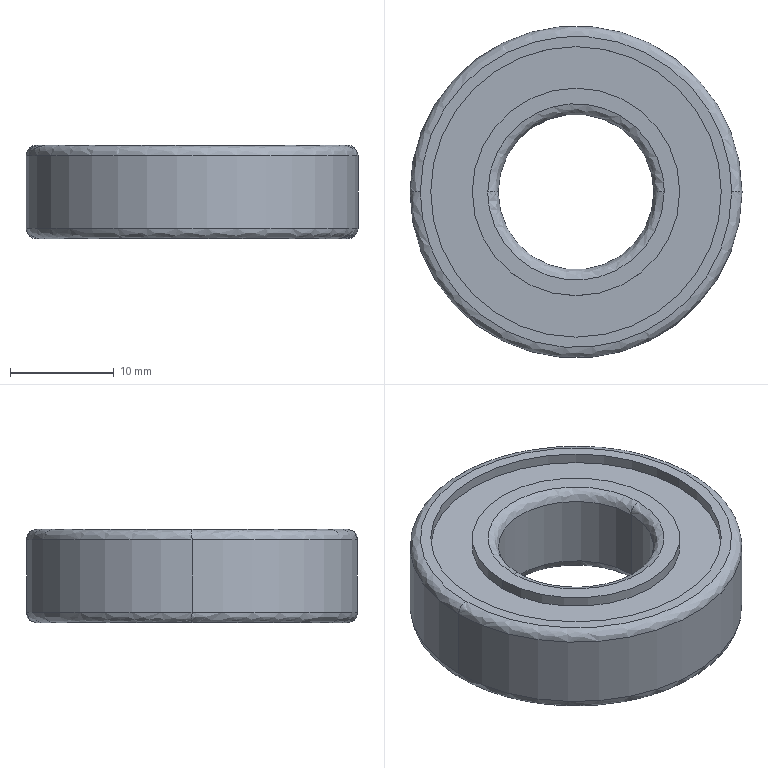Part | STEP file | 6002 | 1 solid | 26 faces | box 32 x 32 x 9 mm | volume 4982 mm3 | cylinder 12 | spline 8 | plane 6 | commonest cylinder face diameters 20 x4 28 x4 15 x2 32 x2